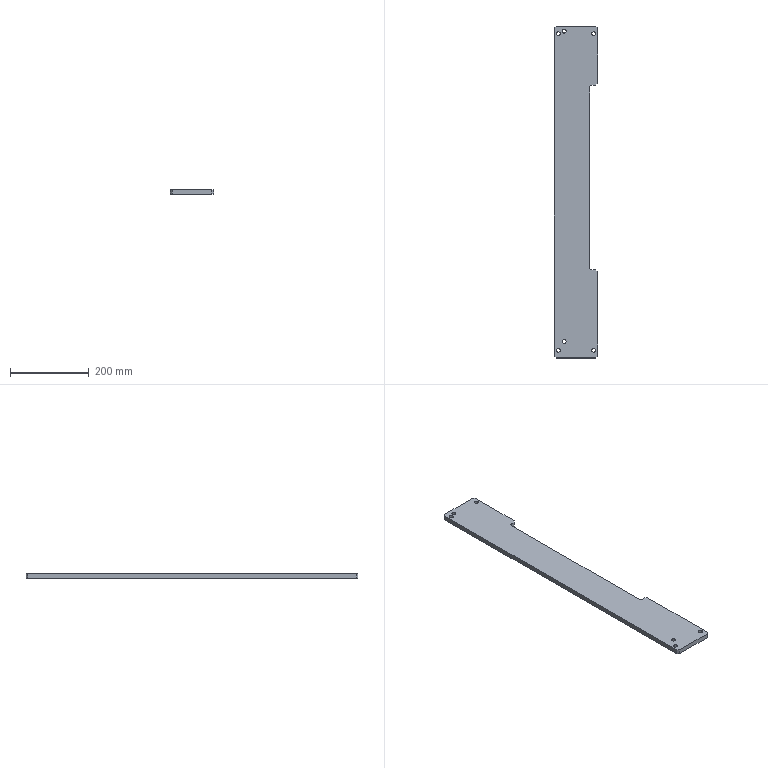Part | STEP file | [10] | 1 solid | 30 faces | box 110 x 844 x 12 mm | volume 994854 mm3 | plane 16 | cylinder 14 | commonest cylinder face diameters 10 x14
STEP:
#1=CARTESIAN_POINT('',(20.,-727.,0.));
#2=VERTEX_POINT('',#1);
#3=CARTESIAN_POINT('',(30.,-727.,0.));
#4=VERTEX_POINT('',#3);
#5=CARTESIAN_POINT('',(25.,-727.,0.));
#6=DIRECTION('',(0.,0.,1.));
#7=DIRECTION('',(1.,0.,0.));
#8=AXIS2_PLACEMENT_3D('',#5,#6,#7);
#9=CIRCLE('',#8,5.);
#10=EDGE_CURVE('',#2,#4,#9,.T.);
#11=ORIENTED_EDGE('',*,*,#10,.F.);
#12=CARTESIAN_POINT('',(20.,-727.,12.));
#13=VERTEX_POINT('',#12);
#14=CARTESIAN_POINT('',(20.,-727.,0.));
#15=DIRECTION('',(0.,0.,1.));
#16=VECTOR('',#15,1000.);
#17=LINE('',#14,#16);
#18=EDGE_CURVE('',#2,#13,#17,.T.);
#19=ORIENTED_EDGE('',*,*,#18,.T.);
#20=CARTESIAN_POINT('',(30.,-727.,12.));
#21=VERTEX_POINT('',#20);
#22=CARTESIAN_POINT('',(25.,-727.,12.));
#23=DIRECTION('',(0.,0.,-1.));
#24=DIRECTION('',(-1.,0.,0.));
#25=AXIS2_PLACEMENT_3D('',#22,#23,#24);
#26=CIRCLE('',#25,5.);
#27=EDGE_CURVE('',#21,#13,#26,.T.);
#28=ORIENTED_EDGE('',*,*,#27,.F.);
#29=CARTESIAN_POINT('',(30.,-727.,0.));
#30=DIRECTION('',(0.,0.,1.));
#31=VECTOR('',#30,1000.);
#32=LINE('',#29,#31);
#33=EDGE_CURVE('',#4,#21,#32,.T.);
#34=ORIENTED_EDGE('',*,*,#33,.F.);
#35=EDGE_LOOP('',(#11,#19,#28,#34));
#36=FACE_OUTER_BOUND('',#35,.T.);
#37=CARTESIAN_POINT('',(25.,-727.,0.));
#38=DIRECTION('',(0.,0.,1.));
#39=DIRECTION('',(1.,0.,0.));
#40=AXIS2_PLACEMENT_3D('',#37,#38,#39);
#41=CYLINDRICAL_SURFACE('',#40,5.);
#42=ADVANCED_FACE('',(#36),#41,.F.);
#43=CARTESIAN_POINT('',(5.,-749.5,0.));
#44=VERTEX_POINT('',#43);
#45=CARTESIAN_POINT('',(15.,-749.5,0.));
#46=VERTEX_POINT('',#45);
#47=CARTESIAN_POINT('',(10.,-749.5,0.));
#48=DIRECTION('',(0.,0.,1.));
#49=DIRECTION('',(1.,0.,0.));
#50=AXIS2_PLACEMENT_3D('',#47,#48,#49);
#51=CIRCLE('',#50,5.);
#52=EDGE_CURVE('',#44,#46,#51,.T.);
#53=ORIENTED_EDGE('',*,*,#52,.F.);
#54=CARTESIAN_POINT('',(5.,-749.5,12.));
#55=VERTEX_POINT('',#54);
#56=CARTESIAN_POINT('',(5.,-749.5,0.));
#57=DIRECTION('',(0.,0.,1.));
#58=VECTOR('',#57,1000.);
#59=LINE('',#56,#58);
#60=EDGE_CURVE('',#44,#55,#59,.T.);
#61=ORIENTED_EDGE('',*,*,#60,.T.);
#62=CARTESIAN_POINT('',(15.,-749.5,12.));
#63=VERTEX_POINT('',#62);
#64=CARTESIAN_POINT('',(10.,-749.5,12.));
#65=DIRECTION('',(0.,0.,-1.));
#66=DIRECTION('',(-1.,0.,0.));
#67=AXIS2_PLACEMENT_3D('',#64,#65,#66);
#68=CIRCLE('',#67,5.);
#69=EDGE_CURVE('',#63,#55,#68,.T.);
#70=ORIENTED_EDGE('',*,*,#69,.F.);
#71=CARTESIAN_POINT('',(15.,-749.5,0.));
#72=DIRECTION('',(0.,0.,1.));
#73=VECTOR('',#72,1000.);
#74=LINE('',#71,#73);
#75=EDGE_CURVE('',#46,#63,#74,.T.);
#76=ORIENTED_EDGE('',*,*,#75,.F.);
#77=EDGE_LOOP('',(#53,#61,#70,#76));
#78=FACE_OUTER_BOUND('',#77,.T.);
#79=CARTESIAN_POINT('',(10.,-749.5,0.));
#80=DIRECTION('',(0.,0.,1.));
#81=DIRECTION('',(1.,0.,0.));
#82=AXIS2_PLACEMENT_3D('',#79,#80,#81);
#83=CYLINDRICAL_SURFACE('',#82,5.);
#84=ADVANCED_FACE('',(#78),#83,.F.);
#85=CARTESIAN_POINT('',(95.,-749.5,0.));
#86=VERTEX_POINT('',#85);
#87=CARTESIAN_POINT('',(105.,-749.5,0.));
#88=VERTEX_POINT('',#87);
#89=CARTESIAN_POINT('',(100.,-749.5,0.));
#90=DIRECTION('',(0.,0.,1.));
#91=DIRECTION('',(1.,0.,0.));
#92=AXIS2_PLACEMENT_3D('',#89,#90,#91);
#93=CIRCLE('',#92,5.);
#94=EDGE_CURVE('',#86,#88,#93,.T.);
#95=ORIENTED_EDGE('',*,*,#94,.F.);
#96=CARTESIAN_POINT('',(95.,-749.5,12.));
#97=VERTEX_POINT('',#96);
#98=CARTESIAN_POINT('',(95.,-749.5,0.));
#99=DIRECTION('',(0.,0.,1.));
#100=VECTOR('',#99,1000.);
#101=LINE('',#98,#100);
#102=EDGE_CURVE('',#86,#97,#101,.T.);
#103=ORIENTED_EDGE('',*,*,#102,.T.);
#104=CARTESIAN_POINT('',(105.,-749.5,12.));
#105=VERTEX_POINT('',#104);
#106=CARTESIAN_POINT('',(100.,-749.5,12.));
#107=DIRECTION('',(0.,0.,-1.));
#108=DIRECTION('',(-1.,0.,0.));
#109=AXIS2_PLACEMENT_3D('',#106,#107,#108);
#110=CIRCLE('',#109,5.);
#111=EDGE_CURVE('',#105,#97,#110,.T.);
#112=ORIENTED_EDGE('',*,*,#111,.F.);
#113=CARTESIAN_POINT('',(105.,-749.5,0.));
#114=DIRECTION('',(0.,0.,1.));
#115=VECTOR('',#114,1000.);
#116=LINE('',#113,#115);
#117=EDGE_CURVE('',#88,#105,#116,.T.);
#118=ORIENTED_EDGE('',*,*,#117,.F.);
#119=EDGE_LOOP('',(#95,#103,#112,#118));
#120=FACE_OUTER_BOUND('',#119,.T.);
#121=CARTESIAN_POINT('',(100.,-749.5,0.));
#122=DIRECTION('',(0.,0.,1.));
#123=DIRECTION('',(1.,0.,0.));
#124=AXIS2_PLACEMENT_3D('',#121,#122,#123);
#125=CYLINDRICAL_SURFACE('',#124,5.);
#126=ADVANCED_FACE('',(#120),#125,.F.);
#127=CARTESIAN_POINT('',(20.,62.,0.));
#128=VERTEX_POINT('',#127);
#129=CARTESIAN_POINT('',(30.,62.,0.));
#130=VERTEX_POINT('',#129);
#131=CARTESIAN_POINT('',(25.,62.,0.));
#132=DIRECTION('',(0.,0.,1.));
#133=DIRECTION('',(1.,0.,0.));
#134=AXIS2_PLACEMENT_3D('',#131,#132,#133);
#135=CIRCLE('',#134,5.);
#136=EDGE_CURVE('',#128,#130,#135,.T.);
#137=ORIENTED_EDGE('',*,*,#136,.F.);
#138=CARTESIAN_POINT('',(20.,62.,12.));
#139=VERTEX_POINT('',#138);
#140=CARTESIAN_POINT('',(20.,62.,0.));
#141=DIRECTION('',(0.,0.,1.));
#142=VECTOR('',#141,1000.);
#143=LINE('',#140,#142);
#144=EDGE_CURVE('',#128,#139,#143,.T.);
#145=ORIENTED_EDGE('',*,*,#144,.T.);
#146=CARTESIAN_POINT('',(30.,62.,12.));
#147=VERTEX_POINT('',#146);
#148=CARTESIAN_POINT('',(25.,62.,12.));
#149=DIRECTION('',(0.,0.,-1.));
#150=DIRECTION('',(-1.,0.,0.));
#151=AXIS2_PLACEMENT_3D('',#148,#149,#150);
#152=CIRCLE('',#151,5.);
#153=EDGE_CURVE('',#147,#139,#152,.T.);
#154=ORIENTED_EDGE('',*,*,#153,.F.);
#155=CARTESIAN_POINT('',(30.,62.,0.));
#156=DIRECTION('',(0.,0.,1.));
#157=VECTOR('',#156,1000.);
#158=LINE('',#155,#157);
#159=EDGE_CURVE('',#130,#147,#158,.T.);
#160=ORIENTED_EDGE('',*,*,#159,.F.);
#161=EDGE_LOOP('',(#137,#145,#154,#160));
#162=FACE_OUTER_BOUND('',#161,.T.);
#163=CARTESIAN_POINT('',(25.,62.,0.));
#164=DIRECTION('',(0.,0.,1.));
#165=DIRECTION('',(1.,0.,0.));
#166=AXIS2_PLACEMENT_3D('',#163,#164,#165);
#167=CYLINDRICAL_SURFACE('',#166,5.);
#168=ADVANCED_FACE('',(#162),#167,.F.);
#169=CARTESIAN_POINT('',(95.,55.5,0.));
#170=VERTEX_POINT('',#169);
#171=CARTESIAN_POINT('',(105.,55.5,0.));
#172=VERTEX_POINT('',#171);
#173=CARTESIAN_POINT('',(100.,55.5,0.));
#174=DIRECTION('',(0.,0.,1.));
#175=DIRECTION('',(1.,0.,0.));
#176=AXIS2_PLACEMENT_3D('',#173,#174,#175);
#177=CIRCLE('',#176,5.);
#178=EDGE_CURVE('',#170,#172,#177,.T.);
#179=ORIENTED_EDGE('',*,*,#178,.F.);
#180=CARTESIAN_POINT('',(95.,55.5,12.));
#181=VERTEX_POINT('',#180);
#182=CARTESIAN_POINT('',(95.,55.5,0.));
#183=DIRECTION('',(0.,0.,1.));
#184=VECTOR('',#183,1000.);
#185=LINE('',#182,#184);
#186=EDGE_CURVE('',#170,#181,#185,.T.);
#187=ORIENTED_EDGE('',*,*,#186,.T.);
#188=CARTESIAN_POINT('',(105.,55.5,12.));
#189=VERTEX_POINT('',#188);
#190=CARTESIAN_POINT('',(100.,55.5,12.));
#191=DIRECTION('',(0.,0.,-1.));
#192=DIRECTION('',(-1.,0.,0.));
#193=AXIS2_PLACEMENT_3D('',#190,#191,#192);
#194=CIRCLE('',#193,5.);
#195=EDGE_CURVE('',#189,#181,#194,.T.);
#196=ORIENTED_EDGE('',*,*,#195,.F.);
#197=CARTESIAN_POINT('',(105.,55.5,0.));
#198=DIRECTION('',(0.,0.,1.));
#199=VECTOR('',#198,1000.);
#200=LINE('',#197,#199);
#201=EDGE_CURVE('',#172,#189,#200,.T.);
#202=ORIENTED_EDGE('',*,*,#201,.F.);
#203=EDGE_LOOP('',(#179,#187,#196,#202));
#204=FACE_OUTER_BOUND('',#203,.T.);
#205=CARTESIAN_POINT('',(100.,55.5,0.));
#206=DIRECTION('',(0.,0.,1.));
#207=DIRECTION('',(1.,0.,0.));
#208=AXIS2_PLACEMENT_3D('',#205,#206,#207);
#209=CYLINDRICAL_SURFACE('',#208,5.);
#210=ADVANCED_FACE('',(#204),#209,.F.);
#211=CARTESIAN_POINT('',(5.,55.5,0.));
#212=VERTEX_POINT('',#211);
#213=CARTESIAN_POINT('',(15.,55.5,0.));
#214=VERTEX_POINT('',#213);
#215=CARTESIAN_POINT('',(10.,55.5,0.));
#216=DIRECTION('',(0.,0.,1.));
#217=DIRECTION('',(1.,0.,0.));
#218=AXIS2_PLACEMENT_3D('',#215,#216,#217);
#219=CIRCLE('',#218,5.);
#220=EDGE_CURVE('',#212,#214,#219,.T.);
#221=ORIENTED_EDGE('',*,*,#220,.F.);
#222=CARTESIAN_POINT('',(5.,55.5,12.));
#223=VERTEX_POINT('',#222);
#224=CARTESIAN_POINT('',(5.,55.5,0.));
#225=DIRECTION('',(0.,0.,1.));
#226=VECTOR('',#225,1000.);
#227=LINE('',#224,#226);
#228=EDGE_CURVE('',#212,#223,#227,.T.);
#229=ORIENTED_EDGE('',*,*,#228,.T.);
#230=CARTESIAN_POINT('',(15.,55.5,12.));
#231=VERTEX_POINT('',#230);
#232=CARTESIAN_POINT('',(10.,55.5,12.));
#233=DIRECTION('',(0.,0.,-1.));
#234=DIRECTION('',(-1.,0.,0.));
#235=AXIS2_PLACEMENT_3D('',#232,#233,#234);
#236=CIRCLE('',#235,5.);
#237=EDGE_CURVE('',#231,#223,#236,.T.);
#238=ORIENTED_EDGE('',*,*,#237,.F.);
#239=CARTESIAN_POINT('',(15.,55.5,0.));
#240=DIRECTION('',(0.,0.,1.));
#241=VECTOR('',#240,1000.);
#242=LINE('',#239,#241);
#243=EDGE_CURVE('',#214,#231,#242,.T.);
#244=ORIENTED_EDGE('',*,*,#243,.F.);
#245=EDGE_LOOP('',(#221,#229,#238,#244));
#246=FACE_OUTER_BOUND('',#245,.T.);
#247=CARTESIAN_POINT('',(10.,55.5,0.));
#248=DIRECTION('',(0.,0.,1.));
#249=DIRECTION('',(1.,0.,0.));
#250=AXIS2_PLACEMENT_3D('',#247,#248,#249);
#251=CYLINDRICAL_SURFACE('',#250,5.);
#252=ADVANCED_FACE('',(#246),#251,.F.);
#253=CARTESIAN_POINT('',(110.,70.,12.));
#254=VERTEX_POINT('',#253);
#255=CARTESIAN_POINT('',(110.,-70.,12.));
#256=VERTEX_POINT('',#255);
#257=CARTESIAN_POINT('',(110.,37.5,12.));
#258=DIRECTION('',(0.,-1.,0.));
#259=VECTOR('',#258,1000.);
#260=LINE('',#257,#259);
#261=EDGE_CURVE('',#254,#256,#260,.T.);
#262=ORIENTED_EDGE('',*,*,#261,.T.);
#263=CARTESIAN_POINT('',(110.,-70.,0.));
#264=VERTEX_POINT('',#263);
#265=CARTESIAN_POINT('',(110.,-70.,0.));
#266=DIRECTION('',(0.,0.,-1.));
#267=VECTOR('',#266,1000.);
#268=LINE('',#265,#267);
#269=EDGE_CURVE('',#256,#264,#268,.T.);
#270=ORIENTED_EDGE('',*,*,#269,.T.);
#271=CARTESIAN_POINT('',(110.,70.,0.));
#272=VERTEX_POINT('',#271);
#273=CARTESIAN_POINT('',(110.,37.5,0.));
#274=DIRECTION('',(0.,1.,0.));
#275=VECTOR('',#274,1000.);
#276=LINE('',#273,#275);
#277=EDGE_CURVE('',#264,#272,#276,.T.);
#278=ORIENTED_EDGE('',*,*,#277,.T.);
#279=CARTESIAN_POINT('',(110.,70.,12.));
#280=DIRECTION('',(0.,0.,1.));
#281=VECTOR('',#280,1000.);
#282=LINE('',#279,#281);
#283=EDGE_CURVE('',#272,#254,#282,.T.);
#284=ORIENTED_EDGE('',*,*,#283,.T.);
#285=EDGE_LOOP('',(#262,#270,#278,#284));
#286=FACE_OUTER_BOUND('',#285,.T.);
#287=CARTESIAN_POINT('',(110.,37.5,12.));
#288=DIRECTION('',(1.,0.,0.));
#289=DIRECTION('',(0.,0.,-1.));
#290=AXIS2_PLACEMENT_3D('',#287,#288,#289);
#291=PLANE('',#290);
#292=ADVANCED_FACE('',(#286),#291,.T.);
#293=CARTESIAN_POINT('',(25.,62.,0.));
#294=DIRECTION('',(0.,0.,1.));
#295=DIRECTION('',(1.,0.,0.));
#296=AXIS2_PLACEMENT_3D('',#293,#294,#295);
#297=CIRCLE('',#296,5.);
#298=EDGE_CURVE('',#130,#128,#297,.T.);
#299=ORIENTED_EDGE('',*,*,#298,.T.);
#300=ORIENTED_EDGE('',*,*,#136,.T.);
#301=EDGE_LOOP('',(#299,#300));
#302=FACE_BOUND('',#301,.T.);
#303=CARTESIAN_POINT('',(100.,55.5,0.));
#304=DIRECTION('',(0.,0.,1.));
#305=DIRECTION('',(1.,0.,0.));
#306=AXIS2_PLACEMENT_3D('',#303,#304,#305);
#307=CIRCLE('',#306,5.);
#308=EDGE_CURVE('',#172,#170,#307,.T.);
#309=ORIENTED_EDGE('',*,*,#308,.T.);
#310=ORIENTED_EDGE('',*,*,#178,.T.);
#311=EDGE_LOOP('',(#309,#310));
#312=FACE_BOUND('',#311,.T.);
#313=CARTESIAN_POINT('',(10.,55.5,0.));
#314=DIRECTION('',(0.,0.,1.));
#315=DIRECTION('',(1.,0.,0.));
#316=AXIS2_PLACEMENT_3D('',#313,#314,#315);
#317=CIRCLE('',#316,5.);
#318=EDGE_CURVE('',#214,#212,#317,.T.);
#319=ORIENTED_EDGE('',*,*,#318,.T.);
#320=ORIENTED_EDGE('',*,*,#220,.T.);
#321=EDGE_LOOP('',(#319,#320));
#322=FACE_BOUND('',#321,.T.);
#323=CARTESIAN_POINT('',(25.,-727.,0.));
#324=DIRECTION('',(0.,0.,1.));
#325=DIRECTION('',(1.,0.,0.));
#326=AXIS2_PLACEMENT_3D('',#323,#324,#325);
#327=CIRCLE('',#326,5.);
#328=EDGE_CURVE('',#4,#2,#327,.T.);
#329=ORIENTED_EDGE('',*,*,#328,.T.);
#330=ORIENTED_EDGE('',*,*,#10,.T.);
#331=EDGE_LOOP('',(#329,#330));
#332=FACE_BOUND('',#331,.T.);
#333=CARTESIAN_POINT('',(10.,-749.5,0.));
#334=DIRECTION('',(0.,0.,1.));
#335=DIRECTION('',(1.,0.,0.));
#336=AXIS2_PLACEMENT_3D('',#333,#334,#335);
#337=CIRCLE('',#336,5.);
#338=EDGE_CURVE('',#46,#44,#337,.T.);
#339=ORIENTED_EDGE('',*,*,#338,.T.);
#340=ORIENTED_EDGE('',*,*,#52,.T.);
#341=EDGE_LOOP('',(#339,#340));
#342=FACE_BOUND('',#341,.T.);
#343=CARTESIAN_POINT('',(100.,-749.5,0.));
#344=DIRECTION('',(0.,0.,1.));
#345=DIRECTION('',(1.,0.,0.));
#346=AXIS2_PLACEMENT_3D('',#343,#344,#345);
#347=CIRCLE('',#346,5.);
#348=EDGE_CURVE('',#88,#86,#347,.T.);
#349=ORIENTED_EDGE('',*,*,#348,.T.);
#350=ORIENTED_EDGE('',*,*,#94,.T.);
#351=EDGE_LOOP('',(#349,#350));
#352=FACE_BOUND('',#351,.T.);
#353=ORIENTED_EDGE('',*,*,#277,.F.);
#354=CARTESIAN_POINT('',(105.,-75.,0.));
#355=VERTEX_POINT('',#354);
#356=CARTESIAN_POINT('',(136.25,-43.75,0.));
#357=DIRECTION('',(-0.7071,-0.7071,0.));
#358=VECTOR('',#357,1000.);
#359=LINE('',#356,#358);
#360=EDGE_CURVE('',#264,#355,#359,.T.);
#361=ORIENTED_EDGE('',*,*,#360,.T.);
#362=CARTESIAN_POINT('',(95.,-75.,0.));
#363=VERTEX_POINT('',#362);
#364=CARTESIAN_POINT('',(100.,-75.,0.));
#365=DIRECTION('',(-1.,0.,0.));
#366=VECTOR('',#365,1000.);
#367=LINE('',#364,#366);
#368=EDGE_CURVE('',#355,#363,#367,.T.);
#369=ORIENTED_EDGE('',*,*,#368,.T.);
#370=CARTESIAN_POINT('',(90.,-80.,0.));
#371=VERTEX_POINT('',#370);
#372=CARTESIAN_POINT('',(95.,-80.,0.));
#373=DIRECTION('',(0.,0.,1.));
#374=DIRECTION('',(-1.,0.,0.));
#375=AXIS2_PLACEMENT_3D('',#372,#373,#374);
#376=CIRCLE('',#375,5.);
#377=EDGE_CURVE('',#363,#371,#376,.T.);
#378=ORIENTED_EDGE('',*,*,#377,.T.);
#379=CARTESIAN_POINT('',(90.,-540.,0.));
#380=VERTEX_POINT('',#379);
#381=CARTESIAN_POINT('',(90.,-310.,0.));
#382=DIRECTION('',(0.,-1.,0.));
#383=VECTOR('',#382,1000.);
#384=LINE('',#381,#383);
#385=EDGE_CURVE('',#371,#380,#384,.T.);
#386=ORIENTED_EDGE('',*,*,#385,.T.);
#387=CARTESIAN_POINT('',(95.,-545.,0.));
#388=VERTEX_POINT('',#387);
#389=CARTESIAN_POINT('',(95.,-540.,0.));
#390=DIRECTION('',(0.,0.,1.));
#391=DIRECTION('',(-1.,0.,0.));
#392=AXIS2_PLACEMENT_3D('',#389,#390,#391);
#393=CIRCLE('',#392,5.);
#394=EDGE_CURVE('',#380,#388,#393,.T.);
#395=ORIENTED_EDGE('',*,*,#394,.T.);
#396=CARTESIAN_POINT('',(105.,-545.,0.));
#397=VERTEX_POINT('',#396);
#398=CARTESIAN_POINT('',(100.,-545.,0.));
#399=DIRECTION('',(1.,0.,0.));
#400=VECTOR('',#399,1000.);
#401=LINE('',#398,#400);
#402=EDGE_CURVE('',#388,#397,#401,.T.);
#403=ORIENTED_EDGE('',*,*,#402,.T.);
#404=CARTESIAN_POINT('',(110.,-550.,0.));
#405=VERTEX_POINT('',#404);
#406=CARTESIAN_POINT('',(-211.25,-228.75,0.));
#407=DIRECTION('',(0.7071,-0.7071,0.));
#408=VECTOR('',#407,1000.);
#409=LINE('',#406,#408);
#410=EDGE_CURVE('',#397,#405,#409,.T.);
#411=ORIENTED_EDGE('',*,*,#410,.T.);
#412=CARTESIAN_POINT('',(110.,-764.,0.));
#413=VERTEX_POINT('',#412);
#414=CARTESIAN_POINT('',(110.,37.5,0.));
#415=DIRECTION('',(0.,1.,0.));
#416=VECTOR('',#415,1000.);
#417=LINE('',#414,#416);
#418=EDGE_CURVE('',#413,#405,#417,.T.);
#419=ORIENTED_EDGE('',*,*,#418,.F.);
#420=CARTESIAN_POINT('',(105.,-769.,0.));
#421=VERTEX_POINT('',#420);
#422=CARTESIAN_POINT('',(272.25,-601.75,0.));
#423=DIRECTION('',(-0.7071,-0.7071,0.));
#424=VECTOR('',#423,1000.);
#425=LINE('',#422,#424);
#426=EDGE_CURVE('',#413,#421,#425,.T.);
#427=ORIENTED_EDGE('',*,*,#426,.T.);
#428=CARTESIAN_POINT('',(5.,-769.,0.));
#429=VERTEX_POINT('',#428);
#430=CARTESIAN_POINT('',(55.,-769.,0.));
#431=DIRECTION('',(1.,0.,0.));
#432=VECTOR('',#431,1000.);
#433=LINE('',#430,#432);
#434=EDGE_CURVE('',#429,#421,#433,.T.);
#435=ORIENTED_EDGE('',*,*,#434,.F.);
#436=CARTESIAN_POINT('',(0.,-764.,0.));
#437=VERTEX_POINT('',#436);
#438=CARTESIAN_POINT('',(-162.25,-601.75,0.));
#439=DIRECTION('',(-0.7071,0.7071,0.));
#440=VECTOR('',#439,1000.);
#441=LINE('',#438,#440);
#442=EDGE_CURVE('',#429,#437,#441,.T.);
#443=ORIENTED_EDGE('',*,*,#442,.T.);
#444=CARTESIAN_POINT('',(0.,70.,0.));
#445=VERTEX_POINT('',#444);
#446=CARTESIAN_POINT('',(0.,37.5,0.));
#447=DIRECTION('',(0.,-1.,0.));
#448=VECTOR('',#447,1000.);
#449=LINE('',#446,#448);
#450=EDGE_CURVE('',#445,#437,#449,.T.);
#451=ORIENTED_EDGE('',*,*,#450,.F.);
#452=CARTESIAN_POINT('',(5.,75.,0.));
#453=VERTEX_POINT('',#452);
#454=CARTESIAN_POINT('',(11.25,81.25,0.));
#455=DIRECTION('',(0.7071,0.7071,0.));
#456=VECTOR('',#455,1000.);
#457=LINE('',#454,#456);
#458=EDGE_CURVE('',#445,#453,#457,.T.);
#459=ORIENTED_EDGE('',*,*,#458,.T.);
#460=CARTESIAN_POINT('',(105.,75.,0.));
#461=VERTEX_POINT('',#460);
#462=CARTESIAN_POINT('',(55.,75.,0.));
#463=DIRECTION('',(-1.,0.,0.));
#464=VECTOR('',#463,1000.);
#465=LINE('',#462,#464);
#466=EDGE_CURVE('',#461,#453,#465,.T.);
#467=ORIENTED_EDGE('',*,*,#466,.F.);
#468=CARTESIAN_POINT('',(98.75,81.25,0.));
#469=DIRECTION('',(0.7071,-0.7071,0.));
#470=VECTOR('',#469,1000.);
#471=LINE('',#468,#470);
#472=EDGE_CURVE('',#461,#272,#471,.T.);
#473=ORIENTED_EDGE('',*,*,#472,.T.);
#474=EDGE_LOOP('',(#353,#361,#369,#378,#386,#395,#403,#411,#419,#427,#435,#443,#451,#459,#467,#473));
#475=FACE_OUTER_BOUND('',#474,.T.);
#476=CARTESIAN_POINT('',(55.,37.5,0.));
#477=DIRECTION('',(0.,0.,-1.));
#478=DIRECTION('',(-1.,0.,0.));
#479=AXIS2_PLACEMENT_3D('',#476,#477,#478);
#480=PLANE('',#479);
#481=ADVANCED_FACE('',(#302,#312,#322,#332,#342,#352,#475),#480,.T.);
#482=ORIENTED_EDGE('',*,*,#153,.T.);
#483=CARTESIAN_POINT('',(25.,62.,12.));
#484=DIRECTION('',(0.,0.,-1.));
#485=DIRECTION('',(-1.,0.,0.));
#486=AXIS2_PLACEMENT_3D('',#483,#484,#485);
#487=CIRCLE('',#486,5.);
#488=EDGE_CURVE('',#139,#147,#487,.T.);
#489=ORIENTED_EDGE('',*,*,#488,.T.);
#490=EDGE_LOOP('',(#482,#489));
#491=FACE_BOUND('',#490,.T.);
#492=ORIENTED_EDGE('',*,*,#195,.T.);
#493=CARTESIAN_POINT('',(100.,55.5,12.));
#494=DIRECTION('',(0.,0.,-1.));
#495=DIRECTION('',(-1.,0.,0.));
#496=AXIS2_PLACEMENT_3D('',#493,#494,#495);
#497=CIRCLE('',#496,5.);
#498=EDGE_CURVE('',#181,#189,#497,.T.);
#499=ORIENTED_EDGE('',*,*,#498,.T.);
#500=EDGE_LOOP('',(#492,#499));
#501=FACE_BOUND('',#500,.T.);
#502=ORIENTED_EDGE('',*,*,#237,.T.);
#503=CARTESIAN_POINT('',(10.,55.5,12.));
#504=DIRECTION('',(0.,0.,-1.));
#505=DIRECTION('',(-1.,0.,0.));
#506=AXIS2_PLACEMENT_3D('',#503,#504,#505);
#507=CIRCLE('',#506,5.);
#508=EDGE_CURVE('',#223,#231,#507,.T.);
#509=ORIENTED_EDGE('',*,*,#508,.T.);
#510=EDGE_LOOP('',(#502,#509));
#511=FACE_BOUND('',#510,.T.);
#512=ORIENTED_EDGE('',*,*,#27,.T.);
#513=CARTESIAN_POINT('',(25.,-727.,12.));
#514=DIRECTION('',(0.,0.,-1.));
#515=DIRECTION('',(-1.,0.,0.));
#516=AXIS2_PLACEMENT_3D('',#513,#514,#515);
#517=CIRCLE('',#516,5.);
#518=EDGE_CURVE('',#13,#21,#517,.T.);
#519=ORIENTED_EDGE('',*,*,#518,.T.);
#520=EDGE_LOOP('',(#512,#519));
#521=FACE_BOUND('',#520,.T.);
#522=ORIENTED_EDGE('',*,*,#69,.T.);
#523=CARTESIAN_POINT('',(10.,-749.5,12.));
#524=DIRECTION('',(0.,0.,-1.));
#525=DIRECTION('',(-1.,0.,0.));
#526=AXIS2_PLACEMENT_3D('',#523,#524,#525);
#527=CIRCLE('',#526,5.);
#528=EDGE_CURVE('',#55,#63,#527,.T.);
#529=ORIENTED_EDGE('',*,*,#528,.T.);
#530=EDGE_LOOP('',(#522,#529));
#531=FACE_BOUND('',#530,.T.);
#532=ORIENTED_EDGE('',*,*,#111,.T.);
#533=CARTESIAN_POINT('',(100.,-749.5,12.));
#534=DIRECTION('',(0.,0.,-1.));
#535=DIRECTION('',(-1.,0.,0.));
#536=AXIS2_PLACEMENT_3D('',#533,#534,#535);
#537=CIRCLE('',#536,5.);
#538=EDGE_CURVE('',#97,#105,#537,.T.);
#539=ORIENTED_EDGE('',*,*,#538,.T.);
#540=EDGE_LOOP('',(#532,#539));
#541=FACE_BOUND('',#540,.T.);
#542=CARTESIAN_POINT('',(95.,-75.,12.));
#543=VERTEX_POINT('',#542);
#544=CARTESIAN_POINT('',(105.,-75.,12.));
#545=VERTEX_POINT('',#544);
#546=CARTESIAN_POINT('',(100.,-75.,12.));
#547=DIRECTION('',(1.,0.,0.));
#548=VECTOR('',#547,1000.);
#549=LINE('',#546,#548);
#550=EDGE_CURVE('',#543,#545,#549,.T.);
#551=ORIENTED_EDGE('',*,*,#550,.T.);
#552=CARTESIAN_POINT('',(136.25,-43.75,12.));
#553=DIRECTION('',(0.7071,0.7071,0.));
#554=VECTOR('',#553,1000.);
#555=LINE('',#552,#554);
#556=EDGE_CURVE('',#545,#256,#555,.T.);
#557=ORIENTED_EDGE('',*,*,#556,.T.);
#558=ORIENTED_EDGE('',*,*,#261,.F.);
#559=CARTESIAN_POINT('',(105.,75.,12.));
#560=VERTEX_POINT('',#559);
#561=CARTESIAN_POINT('',(98.75,81.25,12.));
#562=DIRECTION('',(-0.7071,0.7071,0.));
#563=VECTOR('',#562,1000.);
#564=LINE('',#561,#563);
#565=EDGE_CURVE('',#254,#560,#564,.T.);
#566=ORIENTED_EDGE('',*,*,#565,.T.);
#567=CARTESIAN_POINT('',(5.,75.,12.));
#568=VERTEX_POINT('',#567);
#569=CARTESIAN_POINT('',(55.,75.,12.));
#570=DIRECTION('',(1.,0.,0.));
#571=VECTOR('',#570,1000.);
#572=LINE('',#569,#571);
#573=EDGE_CURVE('',#568,#560,#572,.T.);
#574=ORIENTED_EDGE('',*,*,#573,.F.);
#575=CARTESIAN_POINT('',(0.,70.,12.));
#576=VERTEX_POINT('',#575);
#577=CARTESIAN_POINT('',(11.25,81.25,12.));
#578=DIRECTION('',(-0.7071,-0.7071,0.));
#579=VECTOR('',#578,1000.);
#580=LINE('',#577,#579);
#581=EDGE_CURVE('',#568,#576,#580,.T.);
#582=ORIENTED_EDGE('',*,*,#581,.T.);
#583=CARTESIAN_POINT('',(0.,-764.,12.));
#584=VERTEX_POINT('',#583);
#585=CARTESIAN_POINT('',(0.,37.5,12.));
#586=DIRECTION('',(0.,1.,0.));
#587=VECTOR('',#586,1000.);
#588=LINE('',#585,#587);
#589=EDGE_CURVE('',#584,#576,#588,.T.);
#590=ORIENTED_EDGE('',*,*,#589,.F.);
#591=CARTESIAN_POINT('',(5.,-769.,12.));
#592=VERTEX_POINT('',#591);
#593=CARTESIAN_POINT('',(-162.25,-601.75,12.));
#594=DIRECTION('',(0.7071,-0.7071,0.));
#595=VECTOR('',#594,1000.);
#596=LINE('',#593,#595);
#597=EDGE_CURVE('',#584,#592,#596,.T.);
#598=ORIENTED_EDGE('',*,*,#597,.T.);
#599=CARTESIAN_POINT('',(105.,-769.,12.));
#600=VERTEX_POINT('',#599);
#601=CARTESIAN_POINT('',(55.,-769.,12.));
#602=DIRECTION('',(-1.,0.,0.));
#603=VECTOR('',#602,1000.);
#604=LINE('',#601,#603);
#605=EDGE_CURVE('',#600,#592,#604,.T.);
#606=ORIENTED_EDGE('',*,*,#605,.F.);
#607=CARTESIAN_POINT('',(110.,-764.,12.));
#608=VERTEX_POINT('',#607);
#609=CARTESIAN_POINT('',(272.25,-601.75,12.));
#610=DIRECTION('',(0.7071,0.7071,0.));
#611=VECTOR('',#610,1000.);
#612=LINE('',#609,#611);
#613=EDGE_CURVE('',#600,#608,#612,.T.);
#614=ORIENTED_EDGE('',*,*,#613,.T.);
#615=CARTESIAN_POINT('',(110.,-550.,12.));
#616=VERTEX_POINT('',#615);
#617=CARTESIAN_POINT('',(110.,37.5,12.));
#618=DIRECTION('',(0.,-1.,0.));
#619=VECTOR('',#618,1000.);
#620=LINE('',#617,#619);
#621=EDGE_CURVE('',#616,#608,#620,.T.);
#622=ORIENTED_EDGE('',*,*,#621,.F.);
#623=CARTESIAN_POINT('',(105.,-545.,12.));
#624=VERTEX_POINT('',#623);
#625=CARTESIAN_POINT('',(-211.25,-228.75,12.));
#626=DIRECTION('',(-0.7071,0.7071,0.));
#627=VECTOR('',#626,1000.);
#628=LINE('',#625,#627);
#629=EDGE_CURVE('',#616,#624,#628,.T.);
#630=ORIENTED_EDGE('',*,*,#629,.T.);
#631=CARTESIAN_POINT('',(95.,-545.,12.));
#632=VERTEX_POINT('',#631);
#633=CARTESIAN_POINT('',(100.,-545.,12.));
#634=DIRECTION('',(-1.,0.,0.));
#635=VECTOR('',#634,1000.);
#636=LINE('',#633,#635);
#637=EDGE_CURVE('',#624,#632,#636,.T.);
#638=ORIENTED_EDGE('',*,*,#637,.T.);
#639=CARTESIAN_POINT('',(90.,-540.,12.));
#640=VERTEX_POINT('',#639);
#641=CARTESIAN_POINT('',(95.,-540.,12.));
#642=DIRECTION('',(0.,0.,-1.));
#643=DIRECTION('',(1.,0.,0.));
#644=AXIS2_PLACEMENT_3D('',#641,#642,#643);
#645=CIRCLE('',#644,5.);
#646=EDGE_CURVE('',#632,#640,#645,.T.);
#647=ORIENTED_EDGE('',*,*,#646,.T.);
#648=CARTESIAN_POINT('',(90.,-80.,12.));
#649=VERTEX_POINT('',#648);
#650=CARTESIAN_POINT('',(90.,-310.,12.));
#651=DIRECTION('',(0.,1.,0.));
#652=VECTOR('',#651,1000.);
#653=LINE('',#650,#652);
#654=EDGE_CURVE('',#640,#649,#653,.T.);
#655=ORIENTED_EDGE('',*,*,#654,.T.);
#656=CARTESIAN_POINT('',(95.,-80.,12.));
#657=DIRECTION('',(0.,0.,-1.));
#658=DIRECTION('',(1.,0.,0.));
#659=AXIS2_PLACEMENT_3D('',#656,#657,#658);
#660=CIRCLE('',#659,5.);
#661=EDGE_CURVE('',#649,#543,#660,.T.);
#662=ORIENTED_EDGE('',*,*,#661,.T.);
#663=EDGE_LOOP('',(#551,#557,#558,#566,#574,#582,#590,#598,#606,#614,#622,#630,#638,#647,#655,#662));
#664=FACE_OUTER_BOUND('',#663,.T.);
#665=CARTESIAN_POINT('',(55.,37.5,12.));
#666=DIRECTION('',(0.,0.,1.));
#667=DIRECTION('',(1.,0.,0.));
#668=AXIS2_PLACEMENT_3D('',#665,#666,#667);
#669=PLANE('',#668);
#670=ADVANCED_FACE('',(#491,#501,#511,#521,#531,#541,#664),#669,.T.);
#671=ORIENTED_EDGE('',*,*,#418,.T.);
#672=CARTESIAN_POINT('',(110.,-550.,12.));
#673=DIRECTION('',(0.,0.,1.));
#674=VECTOR('',#673,1000.);
#675=LINE('',#672,#674);
#676=EDGE_CURVE('',#405,#616,#675,.T.);
#677=ORIENTED_EDGE('',*,*,#676,.T.);
#678=ORIENTED_EDGE('',*,*,#621,.T.);
#679=CARTESIAN_POINT('',(110.,-764.,12.));
#680=DIRECTION('',(0.,0.,-1.));
#681=VECTOR('',#680,1000.);
#682=LINE('',#679,#681);
#683=EDGE_CURVE('',#608,#413,#682,.T.);
#684=ORIENTED_EDGE('',*,*,#683,.T.);
#685=EDGE_LOOP('',(#671,#677,#678,#684));
#686=FACE_OUTER_BOUND('',#685,.T.);
#687=CARTESIAN_POINT('',(110.,37.5,12.));
#688=DIRECTION('',(1.,0.,0.));
#689=DIRECTION('',(0.,0.,-1.));
#690=AXIS2_PLACEMENT_3D('',#687,#688,#689);
#691=PLANE('',#690);
#692=ADVANCED_FACE('',(#686),#691,.T.);
#693=ORIENTED_EDGE('',*,*,#573,.T.);
#694=CARTESIAN_POINT('',(105.,75.,12.));
#695=DIRECTION('',(0.,0.,-1.));
#696=VECTOR('',#695,1000.);
#697=LINE('',#694,#696);
#698=EDGE_CURVE('',#560,#461,#697,.T.);
#699=ORIENTED_EDGE('',*,*,#698,.T.);
#700=ORIENTED_EDGE('',*,*,#466,.T.);
#701=CARTESIAN_POINT('',(5.,75.,12.));
#702=DIRECTION('',(0.,0.,1.));
#703=VECTOR('',#702,1000.);
#704=LINE('',#701,#703);
#705=EDGE_CURVE('',#453,#568,#704,.T.);
#706=ORIENTED_EDGE('',*,*,#705,.T.);
#707=EDGE_LOOP('',(#693,#699,#700,#706));
#708=FACE_OUTER_BOUND('',#707,.T.);
#709=CARTESIAN_POINT('',(55.,75.,12.));
#710=DIRECTION('',(0.,1.,0.));
#711=DIRECTION('',(0.,0.,-1.));
#712=AXIS2_PLACEMENT_3D('',#709,#710,#711);
#713=PLANE('',#712);
#714=ADVANCED_FACE('',(#708),#713,.T.);
#715=ORIENTED_EDGE('',*,*,#589,.T.);
#716=CARTESIAN_POINT('',(0.,70.,12.));
#717=DIRECTION('',(0.,0.,-1.));
#718=VECTOR('',#717,1000.);
#719=LINE('',#716,#718);
#720=EDGE_CURVE('',#576,#445,#719,.T.);
#721=ORIENTED_EDGE('',*,*,#720,.T.);
#722=ORIENTED_EDGE('',*,*,#450,.T.);
#723=CARTESIAN_POINT('',(0.,-764.,12.));
#724=DIRECTION('',(0.,0.,1.));
#725=VECTOR('',#724,1000.);
#726=LINE('',#723,#725);
#727=EDGE_CURVE('',#437,#584,#726,.T.);
#728=ORIENTED_EDGE('',*,*,#727,.T.);
#729=EDGE_LOOP('',(#715,#721,#722,#728));
#730=FACE_OUTER_BOUND('',#729,.T.);
#731=CARTESIAN_POINT('',(0.,37.5,12.));
#732=DIRECTION('',(-1.,0.,0.));
#733=DIRECTION('',(0.,0.,1.));
#734=AXIS2_PLACEMENT_3D('',#731,#732,#733);
#735=PLANE('',#734);
#736=ADVANCED_FACE('',(#730),#735,.T.);
#737=ORIENTED_EDGE('',*,*,#581,.F.);
#738=ORIENTED_EDGE('',*,*,#705,.F.);
#739=ORIENTED_EDGE('',*,*,#458,.F.);
#740=ORIENTED_EDGE('',*,*,#720,.F.);
#741=EDGE_LOOP('',(#737,#738,#739,#740));
#742=FACE_OUTER_BOUND('',#741,.T.);
#743=CARTESIAN_POINT('',(0.,70.,12.));
#744=DIRECTION('',(0.7071,-0.7071,0.));
#745=DIRECTION('',(0.,0.,-1.));
#746=AXIS2_PLACEMENT_3D('',#743,#744,#745);
#747=PLANE('',#746);
#748=ADVANCED_FACE('',(#742),#747,.F.);
#749=ORIENTED_EDGE('',*,*,#565,.F.);
#750=ORIENTED_EDGE('',*,*,#283,.F.);
#751=ORIENTED_EDGE('',*,*,#472,.F.);
#752=ORIENTED_EDGE('',*,*,#698,.F.);
#753=EDGE_LOOP('',(#749,#750,#751,#752));
#754=FACE_OUTER_BOUND('',#753,.T.);
#755=CARTESIAN_POINT('',(105.,75.,12.));
#756=DIRECTION('',(-0.7071,-0.7071,0.));
#757=DIRECTION('',(0.,0.,-1.));
#758=AXIS2_PLACEMENT_3D('',#755,#756,#757);
#759=PLANE('',#758);
#760=ADVANCED_FACE('',(#754),#759,.F.);
#761=ORIENTED_EDGE('',*,*,#228,.F.);
#762=ORIENTED_EDGE('',*,*,#318,.F.);
#763=ORIENTED_EDGE('',*,*,#243,.T.);
#764=ORIENTED_EDGE('',*,*,#508,.F.);
#765=EDGE_LOOP('',(#761,#762,#763,#764));
#766=FACE_OUTER_BOUND('',#765,.T.);
#767=CARTESIAN_POINT('',(10.,55.5,0.));
#768=DIRECTION('',(0.,0.,1.));
#769=DIRECTION('',(1.,0.,0.));
#770=AXIS2_PLACEMENT_3D('',#767,#768,#769);
#771=CYLINDRICAL_SURFACE('',#770,5.);
#772=ADVANCED_FACE('',(#766),#771,.F.);
#773=ORIENTED_EDGE('',*,*,#186,.F.);
#774=ORIENTED_EDGE('',*,*,#308,.F.);
#775=ORIENTED_EDGE('',*,*,#201,.T.);
#776=ORIENTED_EDGE('',*,*,#498,.F.);
#777=EDGE_LOOP('',(#773,#774,#775,#776));
#778=FACE_OUTER_BOUND('',#777,.T.);
#779=CARTESIAN_POINT('',(100.,55.5,0.));
#780=DIRECTION('',(0.,0.,1.));
#781=DIRECTION('',(1.,0.,0.));
#782=AXIS2_PLACEMENT_3D('',#779,#780,#781);
#783=CYLINDRICAL_SURFACE('',#782,5.);
#784=ADVANCED_FACE('',(#778),#783,.F.);
#785=ORIENTED_EDGE('',*,*,#144,.F.);
#786=ORIENTED_EDGE('',*,*,#298,.F.);
#787=ORIENTED_EDGE('',*,*,#159,.T.);
#788=ORIENTED_EDGE('',*,*,#488,.F.);
#789=EDGE_LOOP('',(#785,#786,#787,#788));
#790=FACE_OUTER_BOUND('',#789,.T.);
#791=CARTESIAN_POINT('',(25.,62.,0.));
#792=DIRECTION('',(0.,0.,1.));
#793=DIRECTION('',(1.,0.,0.));
#794=AXIS2_PLACEMENT_3D('',#791,#792,#793);
#795=CYLINDRICAL_SURFACE('',#794,5.);
#796=ADVANCED_FACE('',(#790),#795,.F.);
#797=ORIENTED_EDGE('',*,*,#434,.T.);
#798=CARTESIAN_POINT('',(105.,-769.,12.));
#799=DIRECTION('',(0.,0.,1.));
#800=VECTOR('',#799,1000.);
#801=LINE('',#798,#800);
#802=EDGE_CURVE('',#421,#600,#801,.T.);
#803=ORIENTED_EDGE('',*,*,#802,.T.);
#804=ORIENTED_EDGE('',*,*,#605,.T.);
#805=CARTESIAN_POINT('',(5.,-769.,12.));
#806=DIRECTION('',(0.,0.,-1.));
#807=VECTOR('',#806,1000.);
#808=LINE('',#805,#807);
#809=EDGE_CURVE('',#592,#429,#808,.T.);
#810=ORIENTED_EDGE('',*,*,#809,.T.);
#811=EDGE_LOOP('',(#797,#803,#804,#810));
#812=FACE_OUTER_BOUND('',#811,.T.);
#813=CARTESIAN_POINT('',(55.,-769.,12.));
#814=DIRECTION('',(0.,-1.,0.));
#815=DIRECTION('',(0.,0.,-1.));
#816=AXIS2_PLACEMENT_3D('',#813,#814,#815);
#817=PLANE('',#816);
#818=ADVANCED_FACE('',(#812),#817,.T.);
#819=ORIENTED_EDGE('',*,*,#613,.F.);
#820=ORIENTED_EDGE('',*,*,#802,.F.);
#821=ORIENTED_EDGE('',*,*,#426,.F.);
#822=ORIENTED_EDGE('',*,*,#683,.F.);
#823=EDGE_LOOP('',(#819,#820,#821,#822));
#824=FACE_OUTER_BOUND('',#823,.T.);
#825=CARTESIAN_POINT('',(110.,-764.,12.));
#826=DIRECTION('',(-0.7071,0.7071,0.));
#827=DIRECTION('',(0.,0.,-1.));
#828=AXIS2_PLACEMENT_3D('',#825,#826,#827);
#829=PLANE('',#828);
#830=ADVANCED_FACE('',(#824),#829,.F.);
#831=ORIENTED_EDGE('',*,*,#597,.F.);
#832=ORIENTED_EDGE('',*,*,#727,.F.);
#833=ORIENTED_EDGE('',*,*,#442,.F.);
#834=ORIENTED_EDGE('',*,*,#809,.F.);
#835=EDGE_LOOP('',(#831,#832,#833,#834));
#836=FACE_OUTER_BOUND('',#835,.T.);
#837=CARTESIAN_POINT('',(5.,-769.,12.));
#838=DIRECTION('',(0.7071,0.7071,0.));
#839=DIRECTION('',(0.,0.,-1.));
#840=AXIS2_PLACEMENT_3D('',#837,#838,#839);
#841=PLANE('',#840);
#842=ADVANCED_FACE('',(#836),#841,.F.);
#843=ORIENTED_EDGE('',*,*,#102,.F.);
#844=ORIENTED_EDGE('',*,*,#348,.F.);
#845=ORIENTED_EDGE('',*,*,#117,.T.);
#846=ORIENTED_EDGE('',*,*,#538,.F.);
#847=EDGE_LOOP('',(#843,#844,#845,#846));
#848=FACE_OUTER_BOUND('',#847,.T.);
#849=CARTESIAN_POINT('',(100.,-749.5,0.));
#850=DIRECTION('',(0.,0.,1.));
#851=DIRECTION('',(1.,0.,0.));
#852=AXIS2_PLACEMENT_3D('',#849,#850,#851);
#853=CYLINDRICAL_SURFACE('',#852,5.);
#854=ADVANCED_FACE('',(#848),#853,.F.);
#855=ORIENTED_EDGE('',*,*,#60,.F.);
#856=ORIENTED_EDGE('',*,*,#338,.F.);
#857=ORIENTED_EDGE('',*,*,#75,.T.);
#858=ORIENTED_EDGE('',*,*,#528,.F.);
#859=EDGE_LOOP('',(#855,#856,#857,#858));
#860=FACE_OUTER_BOUND('',#859,.T.);
#861=CARTESIAN_POINT('',(10.,-749.5,0.));
#862=DIRECTION('',(0.,0.,1.));
#863=DIRECTION('',(1.,0.,0.));
#864=AXIS2_PLACEMENT_3D('',#861,#862,#863);
#865=CYLINDRICAL_SURFACE('',#864,5.);
#866=ADVANCED_FACE('',(#860),#865,.F.);
#867=ORIENTED_EDGE('',*,*,#18,.F.);
#868=ORIENTED_EDGE('',*,*,#328,.F.);
#869=ORIENTED_EDGE('',*,*,#33,.T.);
#870=ORIENTED_EDGE('',*,*,#518,.F.);
#871=EDGE_LOOP('',(#867,#868,#869,#870));
#872=FACE_OUTER_BOUND('',#871,.T.);
#873=CARTESIAN_POINT('',(25.,-727.,0.));
#874=DIRECTION('',(0.,0.,1.));
#875=DIRECTION('',(1.,0.,0.));
#876=AXIS2_PLACEMENT_3D('',#873,#874,#875);
#877=CYLINDRICAL_SURFACE('',#876,5.);
#878=ADVANCED_FACE('',(#872),#877,.F.);
#879=ORIENTED_EDGE('',*,*,#654,.F.);
#880=CARTESIAN_POINT('',(90.,-540.,0.));
#881=DIRECTION('',(0.,0.,-1.));
#882=VECTOR('',#881,1000.);
#883=LINE('',#880,#882);
#884=EDGE_CURVE('',#640,#380,#883,.T.);
#885=ORIENTED_EDGE('',*,*,#884,.T.);
#886=ORIENTED_EDGE('',*,*,#385,.F.);
#887=CARTESIAN_POINT('',(90.,-80.,12.));
#888=DIRECTION('',(0.,0.,1.));
#889=VECTOR('',#888,1000.);
#890=LINE('',#887,#889);
#891=EDGE_CURVE('',#371,#649,#890,.T.);
#892=ORIENTED_EDGE('',*,*,#891,.T.);
#893=EDGE_LOOP('',(#879,#885,#886,#892));
#894=FACE_OUTER_BOUND('',#893,.T.);
#895=CARTESIAN_POINT('',(90.,-310.,12.));
#896=DIRECTION('',(-1.,0.,0.));
#897=DIRECTION('',(0.,0.,1.));
#898=AXIS2_PLACEMENT_3D('',#895,#896,#897);
#899=PLANE('',#898);
#900=ADVANCED_FACE('',(#894),#899,.F.);
#901=ORIENTED_EDGE('',*,*,#637,.F.);
#902=CARTESIAN_POINT('',(105.,-545.,0.));
#903=DIRECTION('',(0.,0.,-1.));
#904=VECTOR('',#903,1000.);
#905=LINE('',#902,#904);
#906=EDGE_CURVE('',#624,#397,#905,.T.);
#907=ORIENTED_EDGE('',*,*,#906,.T.);
#908=ORIENTED_EDGE('',*,*,#402,.F.);
#909=CARTESIAN_POINT('',(95.,-545.,12.));
#910=DIRECTION('',(0.,0.,1.));
#911=VECTOR('',#910,1000.);
#912=LINE('',#909,#911);
#913=EDGE_CURVE('',#388,#632,#912,.T.);
#914=ORIENTED_EDGE('',*,*,#913,.T.);
#915=EDGE_LOOP('',(#901,#907,#908,#914));
#916=FACE_OUTER_BOUND('',#915,.T.);
#917=CARTESIAN_POINT('',(100.,-545.,12.));
#918=DIRECTION('',(0.,-1.,0.));
#919=DIRECTION('',(0.,0.,-1.));
#920=AXIS2_PLACEMENT_3D('',#917,#918,#919);
#921=PLANE('',#920);
#922=ADVANCED_FACE('',(#916),#921,.F.);
#923=ORIENTED_EDGE('',*,*,#368,.F.);
#924=CARTESIAN_POINT('',(105.,-75.,12.));
#925=DIRECTION('',(0.,0.,1.));
#926=VECTOR('',#925,1000.);
#927=LINE('',#924,#926);
#928=EDGE_CURVE('',#355,#545,#927,.T.);
#929=ORIENTED_EDGE('',*,*,#928,.T.);
#930=ORIENTED_EDGE('',*,*,#550,.F.);
#931=CARTESIAN_POINT('',(95.,-75.,0.));
#932=DIRECTION('',(0.,0.,-1.));
#933=VECTOR('',#932,1000.);
#934=LINE('',#931,#933);
#935=EDGE_CURVE('',#543,#363,#934,.T.);
#936=ORIENTED_EDGE('',*,*,#935,.T.);
#937=EDGE_LOOP('',(#923,#929,#930,#936));
#938=FACE_OUTER_BOUND('',#937,.T.);
#939=CARTESIAN_POINT('',(100.,-75.,12.));
#940=DIRECTION('',(0.,1.,0.));
#941=DIRECTION('',(0.,0.,1.));
#942=AXIS2_PLACEMENT_3D('',#939,#940,#941);
#943=PLANE('',#942);
#944=ADVANCED_FACE('',(#938),#943,.F.);
#945=ORIENTED_EDGE('',*,*,#661,.F.);
#946=ORIENTED_EDGE('',*,*,#891,.F.);
#947=ORIENTED_EDGE('',*,*,#377,.F.);
#948=ORIENTED_EDGE('',*,*,#935,.F.);
#949=EDGE_LOOP('',(#945,#946,#947,#948));
#950=FACE_OUTER_BOUND('',#949,.T.);
#951=CARTESIAN_POINT('',(95.,-80.,12.));
#952=DIRECTION('',(0.,0.,1.));
#953=DIRECTION('',(1.,0.,0.));
#954=AXIS2_PLACEMENT_3D('',#951,#952,#953);
#955=CYLINDRICAL_SURFACE('',#954,5.);
#956=ADVANCED_FACE('',(#950),#955,.F.);
#957=ORIENTED_EDGE('',*,*,#646,.F.);
#958=ORIENTED_EDGE('',*,*,#913,.F.);
#959=ORIENTED_EDGE('',*,*,#394,.F.);
#960=ORIENTED_EDGE('',*,*,#884,.F.);
#961=EDGE_LOOP('',(#957,#958,#959,#960));
#962=FACE_OUTER_BOUND('',#961,.T.);
#963=CARTESIAN_POINT('',(95.,-540.,12.));
#964=DIRECTION('',(0.,0.,1.));
#965=DIRECTION('',(1.,0.,0.));
#966=AXIS2_PLACEMENT_3D('',#963,#964,#965);
#967=CYLINDRICAL_SURFACE('',#966,5.);
#968=ADVANCED_FACE('',(#962),#967,.F.);
#969=ORIENTED_EDGE('',*,*,#629,.F.);
#970=ORIENTED_EDGE('',*,*,#676,.F.);
#971=ORIENTED_EDGE('',*,*,#410,.F.);
#972=ORIENTED_EDGE('',*,*,#906,.F.);
#973=EDGE_LOOP('',(#969,#970,#971,#972));
#974=FACE_OUTER_BOUND('',#973,.T.);
#975=CARTESIAN_POINT('',(105.,-545.,12.));
#976=DIRECTION('',(0.7071,0.7071,0.));
#977=DIRECTION('',(0.,0.,1.));
#978=AXIS2_PLACEMENT_3D('',#975,#976,#977);
#979=PLANE('',#978);
#980=ADVANCED_FACE('',(#974),#979,.T.);
#981=ORIENTED_EDGE('',*,*,#556,.F.);
#982=ORIENTED_EDGE('',*,*,#928,.F.);
#983=ORIENTED_EDGE('',*,*,#360,.F.);
#984=ORIENTED_EDGE('',*,*,#269,.F.);
#985=EDGE_LOOP('',(#981,#982,#983,#984));
#986=FACE_OUTER_BOUND('',#985,.T.);
#987=CARTESIAN_POINT('',(110.,-70.,12.));
#988=DIRECTION('',(0.7071,-0.7071,0.));
#989=DIRECTION('',(0.,0.,1.));
#990=AXIS2_PLACEMENT_3D('',#987,#988,#989);
#991=PLANE('',#990);
#992=ADVANCED_FACE('',(#986),#991,.T.);
#993=CLOSED_SHELL('',(#42,#84,#126,#168,#210,#252,#292,#481,#670,#692,#714,#736,#748,#760,#772,#784,#796,#818,#830,#842,#854,#866,#878,#900,#922,#944,#956,#968,#980,#992));
#994=MANIFOLD_SOLID_BREP('',#993);
#995=CARTESIAN_POINT('',(0.,0.,0.));
#996=DIRECTION('',(0.,0.,1.));
#997=DIRECTION('',(1.,0.,0.));
#998=AXIS2_PLACEMENT_3D('',#995,#996,#997);
#999=(LENGTH_UNIT()NAMED_UNIT(*)SI_UNIT(.MILLI.,.METRE.));
#1000=UNCERTAINTY_MEASURE_WITH_UNIT(LENGTH_MEASURE(0.00001),#999,'','');
#1001=(NAMED_UNIT(*)PLANE_ANGLE_UNIT()SI_UNIT($,.RADIAN.));
#1002=(NAMED_UNIT(*)SI_UNIT($,.STERADIAN.)SOLID_ANGLE_UNIT());
#1003=(GEOMETRIC_REPRESENTATION_CONTEXT(3)GLOBAL_UNCERTAINTY_ASSIGNED_CONTEXT((#1000))GLOBAL_UNIT_ASSIGNED_CONTEXT((#999,#1001,#1002))REPRESENTATION_CONTEXT('',''));
#1004=ADVANCED_BREP_SHAPE_REPRESENTATION('',(#994,#998),#1003);